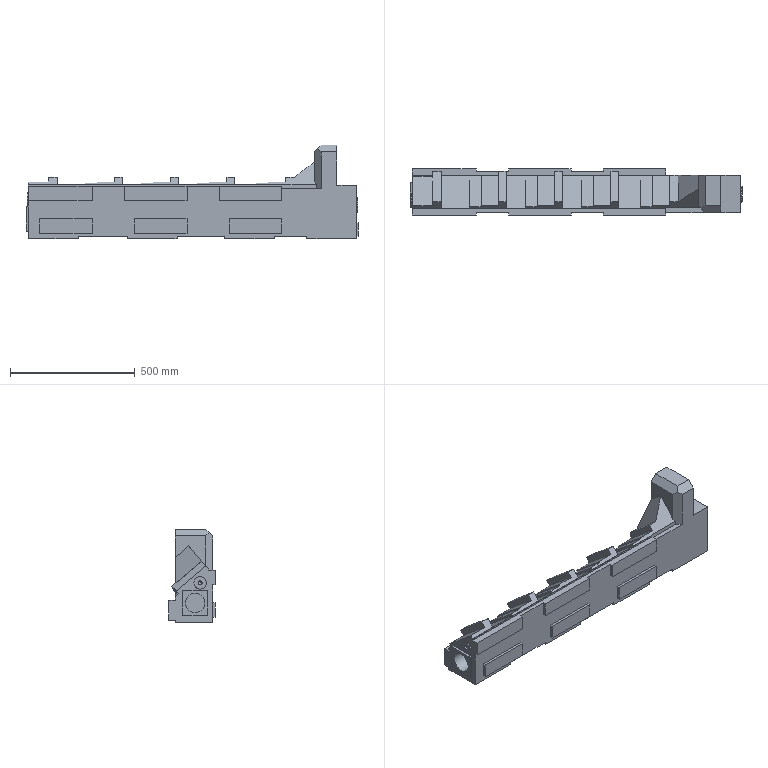Part | NX | features solid 2 | 1 solid | 131 faces | box 1330 x 185 x 375 mm | volume 40194150 mm3 | plane 124 | cylinder 5 | cone 2 | commonest cylinder face diameters 16 x2 50 x1 60 x1 78 x1